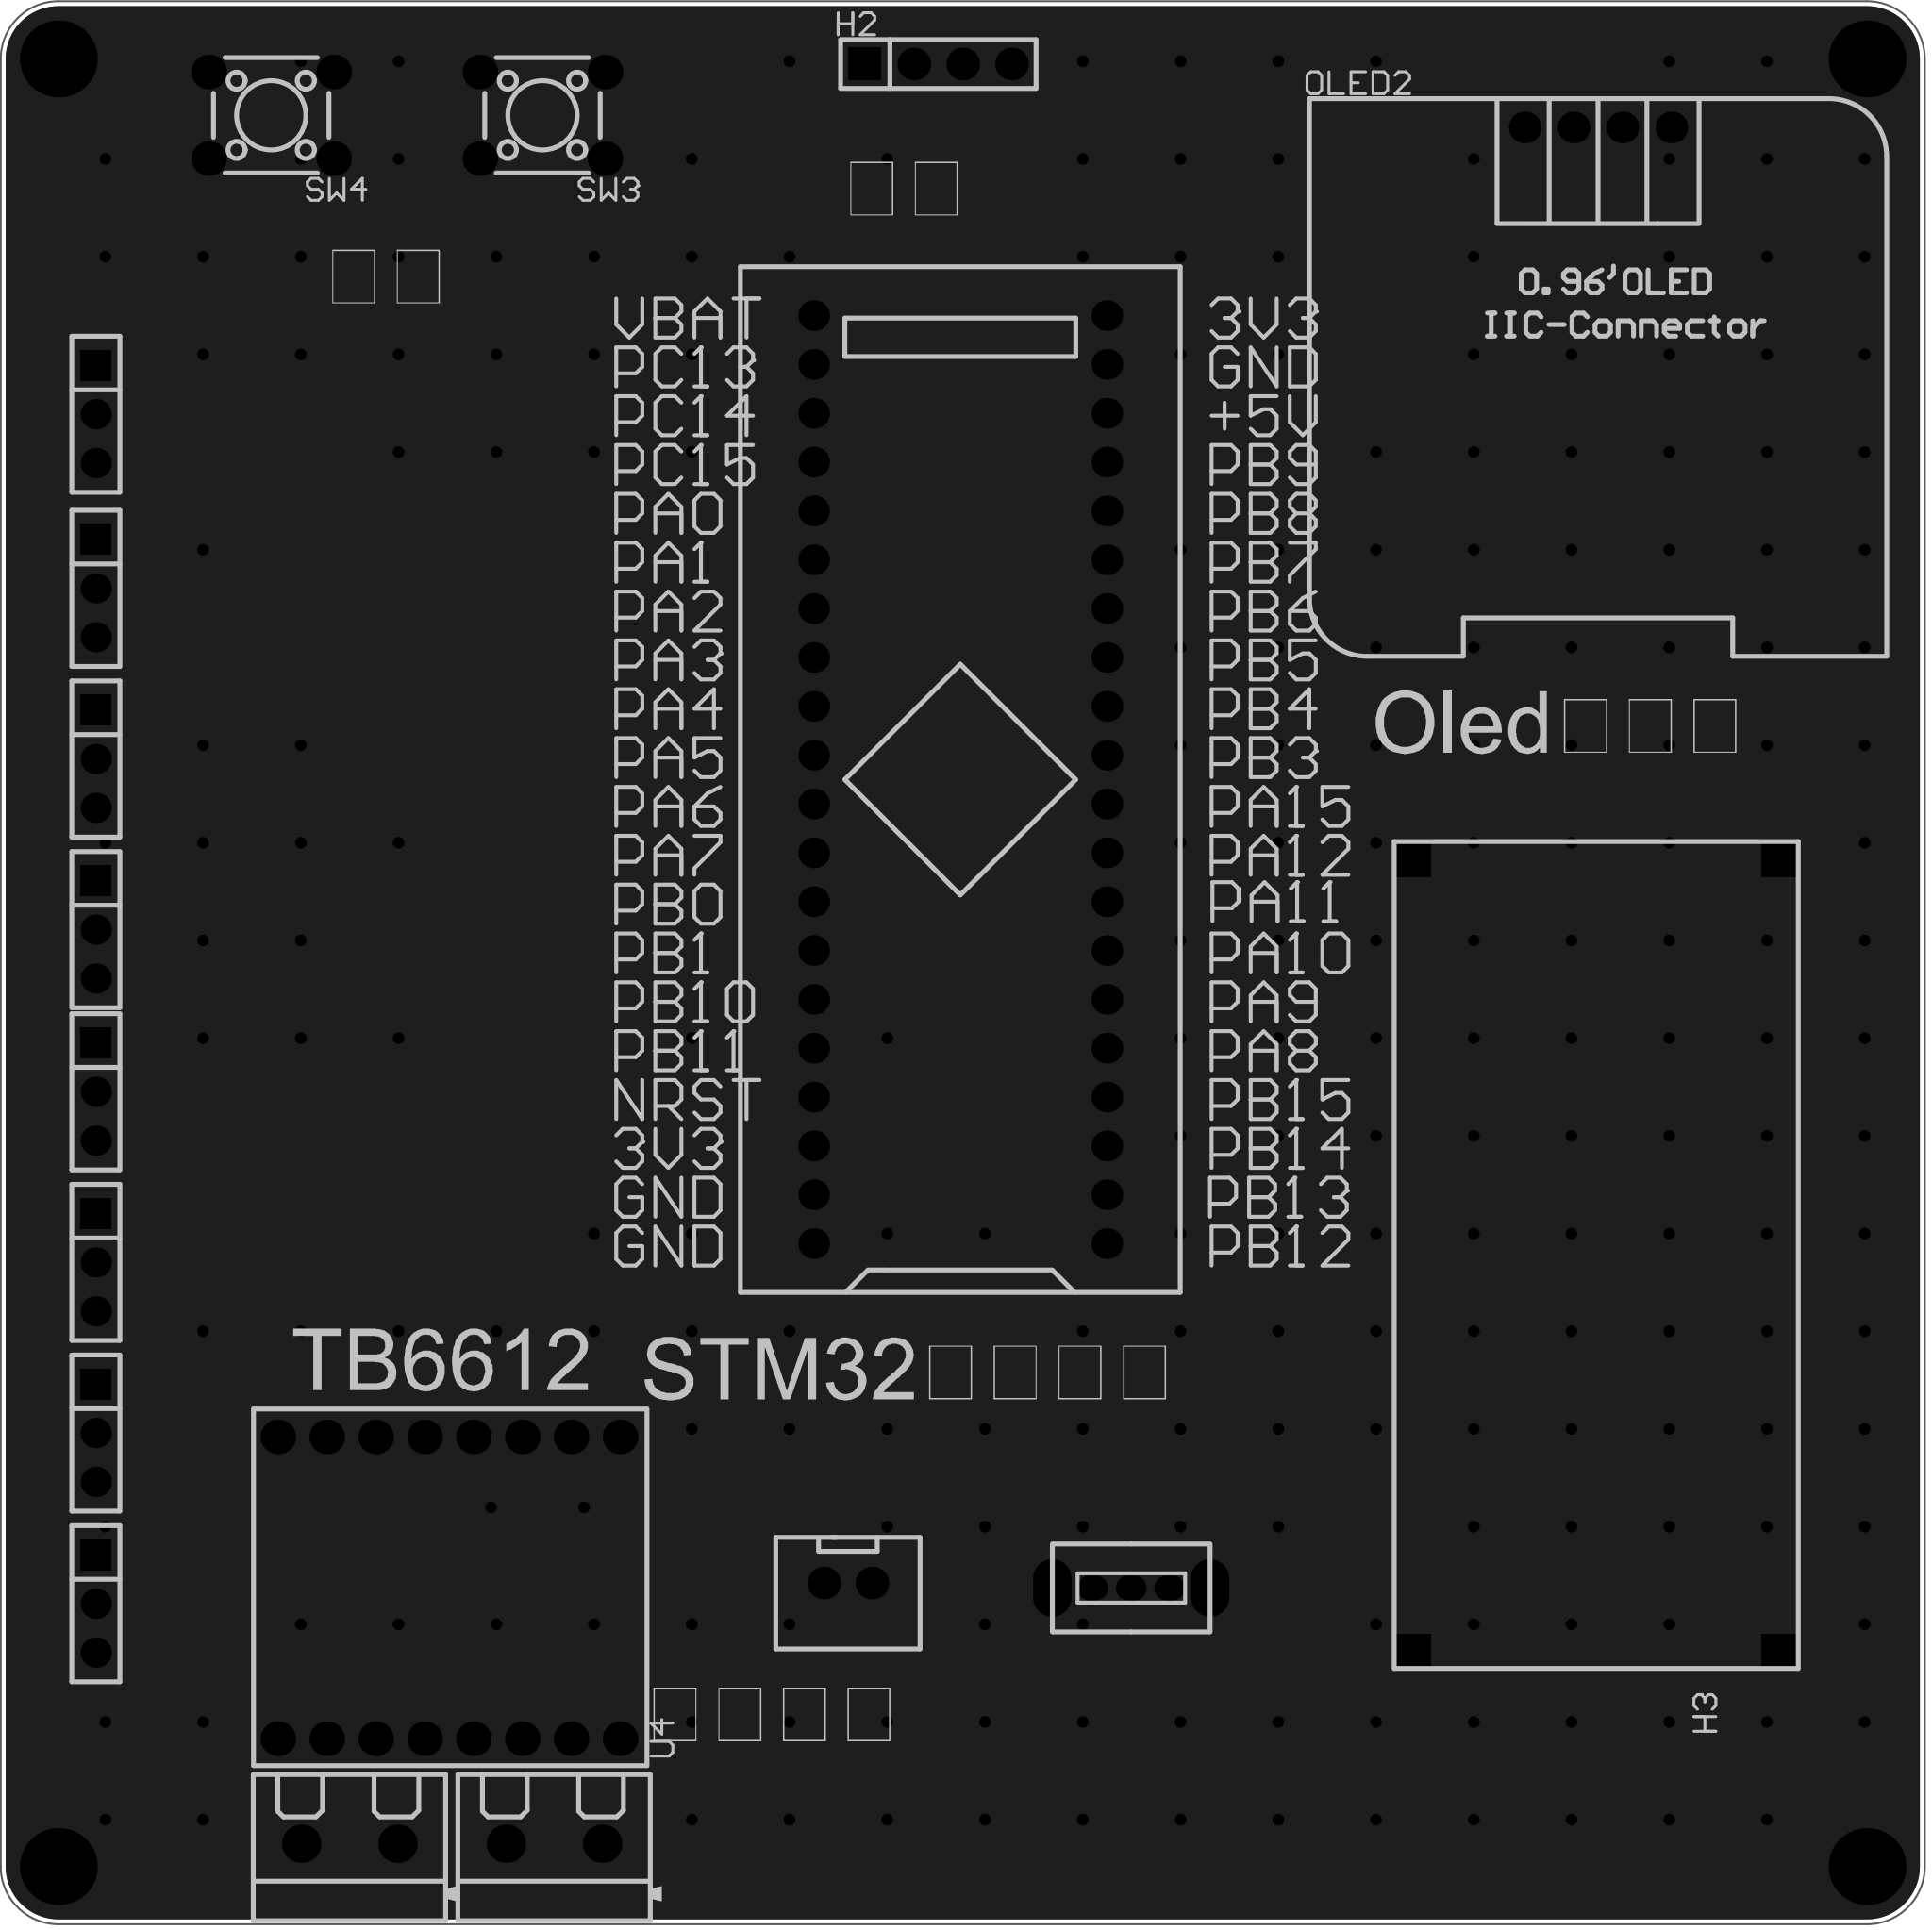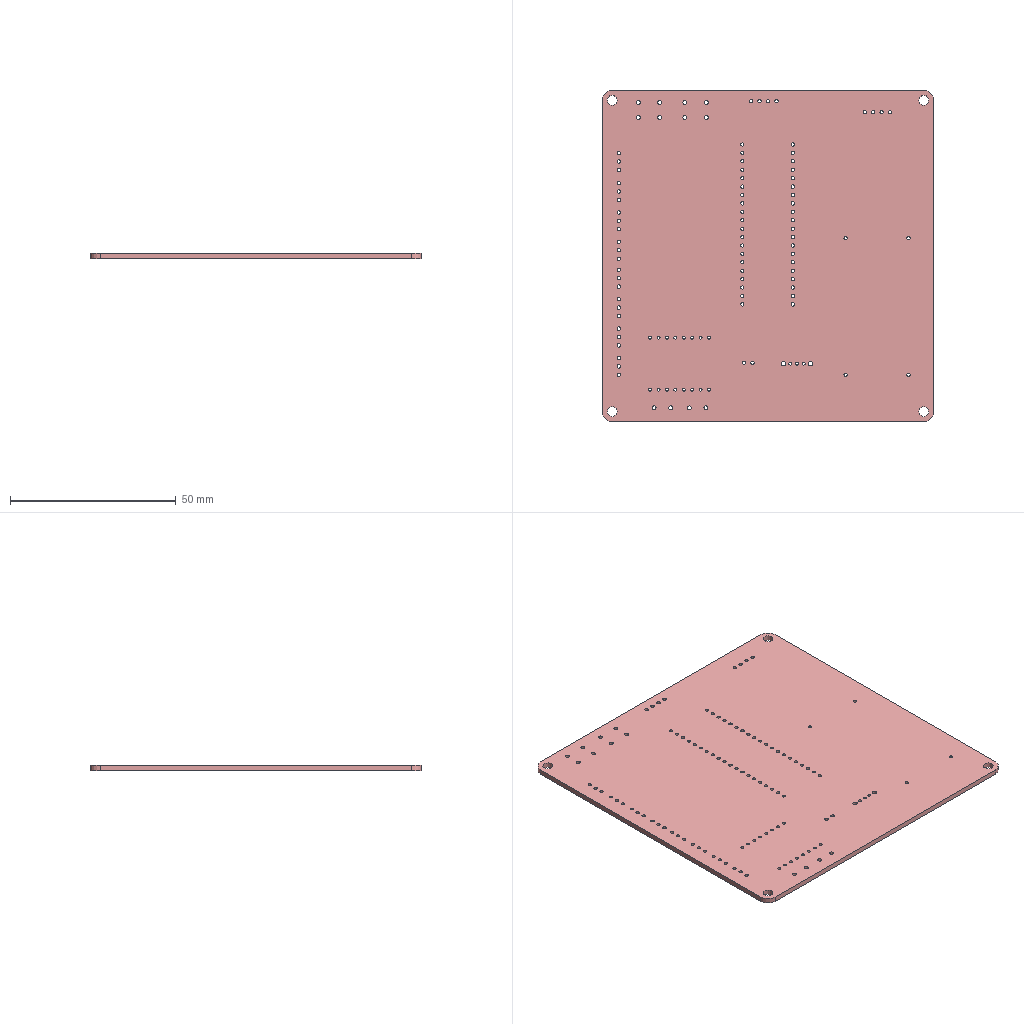Circuit board layout | Altium Designer | box 100 x 100 x 1.6 mm
Layer stack:
# Altium Designer layer stack of  (unit mm; dielectric type: 0 none, 1 core, 2 prepreg, 3 surface material)
index,name,kind,layer,copper_thickness_mm,dielectric_type,dielectric_thickness_mm,dielectric_material,dielectric_constant
0,Top Paste Mask Layer,other,,,,,,
1,Top Silkscreen Layer,other,,,,,,
2,Top Solder Mask Layer,dielectric,,,3,0.01,,3.3
3,Top Layer,copper,Top Layer,0.035,,,,
4,Dielectric1,dielectric,,,3,1.51,FR4,4.5
5,Bottom Layer,copper,Bottom Layer,0.035,,,,
6,Bottom Solder Mask Layer,dielectric,,,3,0.01,,3.3
7,Bottom Silkscreen Layer,other,,,,,,
8,Bottom Paste Mask Layer,other,,,,,,
# drill layer pairs: low layer,high layer
drill_pair,Top Layer,Bottom Layer
Part placement:
Designator,Comment,Layer,Footprint,Center-X(mm),Center-Y(mm),Rotation
U1,STM32F103C8T6-Card,TopLayer,CONN-TH_L53.3-W22.9_STM32F103C8T6-CARD,141.224,140.462,90
SW3,,TopLayer,SW-TH_4P-L6.0-W6.0-P4.50-LS6.5,119.507,175.006,180
SW4,,TopLayer,SW-TH_4P-L6.0-W6.0-P4.50-LS6.5,105.41,175.006,180
CN4,XH2.54*2P_直插,TopLayer,CONN-TH_2P-P2.50-XH2.54-2P,135.382,98.679,0
SW5,,TopLayer,拨动开关,150.106,98.425,180
H6,,TopLayer,HDR-TH_3P-P2.54-V-F,96.293,159.46,270
OLED2,,TopLayer,0.96OLED_4P,174.371,174.371,0
H2,,TopLayer,HDR-TH_4P-P2.54-V-M,140.081,177.673,0
H9,,TopLayer,HDR-TH_3P-P2.54-V-F,96.293,150.405,270
H10,,TopLayer,HDR-TH_3P-P2.54-V-F,96.293,141.531,270
H11,,TopLayer,HDR-TH_3P-P2.54-V-F,96.293,132.657,270
H13,,TopLayer,HDR-TH_3P-P2.54-V-F,96.293,124.227,270
H14,,TopLayer,HDR-TH_3P-P2.54-V-F,96.293,115.353,270
H15,,TopLayer,HDR-TH_3P-P2.54-V-F,96.293,106.479,270
H16,,TopLayer,HDR-TH_3P-P2.54-V-F,96.293,97.605,270
P1,KF301-2P接线端子,TopLayer,CONN-TH_XY301V-A-5.0-2P,109.475,85.121,0
P2,KF301-2P接线端子,TopLayer,CONN-TH_XY301V-A-5.0-2P,120.111,85.121,0
H3,,TopLayer,HDR-TH_4P-P2.54-V-F-R2-C2-S2.54,174.269,115.71,90
U4,,TopLayer,tb6612,114.65,98.431,90
Pad and via stacks:
# Altium Designer via and pad stacks of  (unit mm). Each distinct definition once, with the count of objects using it.
# via: kind,start_layer,end_layer,hole_mm,diameter_mm,mode(0 simple;1 top-mid-bottom;2 full stack),diameter_per_layer,count,example_net
# pad: kind,layer,hole_mm,hole_type(0 round;1 square;2 slot),plating,top_size,top_shape(1 round;2 rect;3 octagon;9 rounded rect),mid_size,bottom_size,mode,footprint,size_per_layer,count,example
pad,Multi-Layer,3,0,plated,4x4,1,4x4,4x4,0,,,4,1
pad,Multi-Layer,1,0,plated,1.6x1.6,1,1.6x1.6,1.6x1.6,0,CONN-TH_L53.3-W22.9_STM32F103C8T6-CARD,,40,U1.1
pad,Multi-Layer,1.2,0,plated,1.8x1.8,1,1.8x1.8,1.8x1.8,0,SW-TH_4P-L6.0-W6.0-P4.50-LS6.5,,8,SW3.1
pad,Multi-Layer,1.05,0,plated,1.7x1.7,1,1.7x1.7,1.7x1.7,0,CONN-TH_2P-P2.50-XH2.54-2P,,2,CN4.2
pad,Multi-Layer,0.8992,0,plated,1.6x1.3,1,1.6x1.3,1.6x1.3,0,\u00B2\u00A6\u00B6\u00AF\u00BF\u00AA\u00B9\u00D8,,3,SW5.1
pad,Multi-Layer,1.3,0,plated,3x1.999,1,3x1.999,3x1.999,0,\u00B2\u00A6\u00B6\u00AF\u00BF\u00AA\u00B9\u00D8,,2,SW5.4
pad,Multi-Layer,1.02,0,plated,1.575x1.575,1,1.575x1.575,1.575x1.575,0,HDR-TH_3P-P2.54-V-F,,16,H6.3
pad,Multi-Layer,1.02,0,plated,1.575x1.575,2,1.575x1.575,1.575x1.575,0,HDR-TH_3P-P2.54-V-F,,8,H6.1
pad,Multi-Layer,1,0,plated,1.65x1.65,1,1.65x1.65,1.65x1.65,0,0.96OLED_4P,,4,OLED2.4
pad,Multi-Layer,1.1,0,plated,1.7x1.7,2,1.7x1.7,1.7x1.7,0,HDR-TH_4P-P2.54-V-M,,1,H2.1
pad,Multi-Layer,1.1,0,plated,1.7x1.7,1,1.7x1.7,1.7x1.7,0,HDR-TH_4P-P2.54-V-M,,3,H2.2
pad,Multi-Layer,1.2,0,plated,2x2,1,2x2,2x2,0,CONN-TH_XY301V-A-5.0-2P,,4,P1.1
pad,Multi-Layer,1,0,plated,1.8x1.8,2,1.8x1.8,1.8x1.8,0,HDR-TH_4P-P2.54-V-F-R2-C2-S2.54,,4,H3.2
pad,Multi-Layer,0.9,0,plated,1.8x1.8,1,1.8x1.8,1.8x1.8,0,tb6612,,16,U4.1
via,Top Layer,Bottom Layer,0.3048,0.61,0,,224,PA0
Copper pours:
name,layer,net,type(0 solid;1 hatched;2 none)
Bottom Layer-GND,Bottom Layer,GND,0
Top Layer-GND,Top Layer,GND,0
Design rules, without the lines most boards share:
# Altium Designer design rules of  (exported by Altium Designer, unit mm)
# columns: name | kind | enabled | priority | scope1 | scope2 | descriptor | typed fields (field=value)
Copper_copperRegion_copperThickness1oz | 0 | disabled | 4 | All | All | Clearance Constraint (Gap=5.984mil) (Disabled)(All),(All) | gap=0.152
Copper_copperRegion_copperThickness1oz_1 | 63 | disabled | 4 | All | All | Board Clearance Constraint (Gap=0mil) (Disabled)(All) |
Copper_copperRegion_Copper_copperRegion | 0 | disabled | 5 | All | All | Clearance Constraint (Gap=5.984mil) (Disabled)(All),(All) | gap=0.152
Copper_copperRegion_Copper_copperRegion_1 | 63 | disabled | 5 | All | All | Board Clearance Constraint (Gap=0mil) (Disabled)(All) |
copperThickness1oz | 0 | enabled | 6 | All | All | Clearance Constraint (Gap=5.984mil) (All),(All) | gap=0.152
copperThickness1oz_1 | 63 | enabled | 6 | All | All | Board Clearance Constraint (Gap=0mil) (All) |
copperRegion_copperThickness1oz | 20 | disabled | 1 | All | All | Polygon Connect Rule(Relief Connect )(Conductor Width=10mil) (Relief Angle=90 Angle) (Entries=4) (Air Gap Width=10mil) (Disabled)(All),(All) | connect_style(0=relief,1=direct,2=none)=0 relief_conductor_width=0.254 relief_entries=4
copperRegion_Copper_copperRegion | 20 | disabled | 2 | All | All | Polygon Connect Rule(Relief Connect )(Conductor Width=10mil) (Relief Angle=90 Angle) (Entries=4) (Air Gap Width=10mil) (Disabled)(All),(All) | connect_style(0=relief,1=direct,2=none)=0 relief_conductor_width=0.254 relief_entries=4
copperRegion | 20 | enabled | 3 | All | All | Polygon Connect Rule(Relief Connect )(Conductor Width=10mil) (Relief Angle=90 Angle) (Entries=4) (Air Gap Width=10mil) (All),(All) | connect_style(0=relief,1=direct,2=none)=0 relief_conductor_width=0.254 relief_entries=4